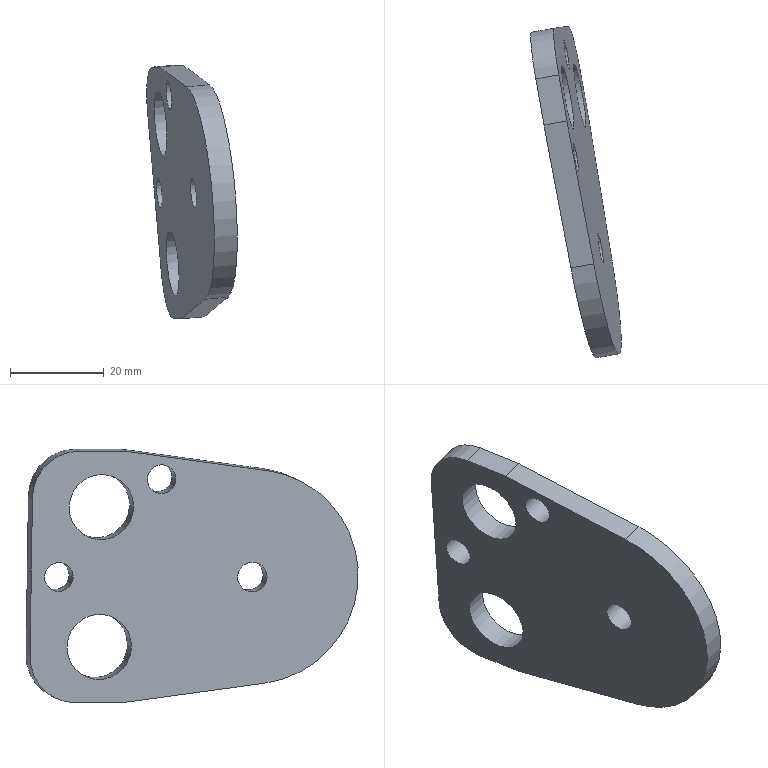Part | NX | features solid 2 | 1 solid | 15 faces | box 19.355 x 71.047 x 54.23 mm | volume 14370 mm3 | cylinder 8 | plane 7 | commonest cylinder face diameters 6.2 x2 14 x2 20 x2 6.4 x1 46 x1
STEP:
#1=CARTESIAN_POINT('',(1568.653,611.082,44.014));
#2=VERTEX_POINT('',#1);
#3=CARTESIAN_POINT('',(1567.775,621.082,34.053));
#4=VERTEX_POINT('',#3);
#5=CARTESIAN_POINT('',(1569.511,611.234,34.053));
#6=DIRECTION('',(-0.9811,-0.173,-0.08716));
#7=DIRECTION('',(-0.1736,0.9848,0.));
#8=AXIS2_PLACEMENT_3D('',#5,#6,#7);
#9=CIRCLE('',#8,10.);
#10=EDGE_CURVE('',#2,#4,#9,.T.);
#11=ORIENTED_EDGE('',*,*,#10,.F.);
#12=CARTESIAN_POINT('',(1573.558,611.947,44.45));
#13=VERTEX_POINT('',#12);
#14=CARTESIAN_POINT('',(1573.558,611.947,44.45));
#15=DIRECTION('',(-0.9811,-0.173,-0.08716));
#16=VECTOR('',#15,1000.);
#17=LINE('',#14,#16);
#18=EDGE_CURVE('',#13,#2,#17,.T.);
#19=ORIENTED_EDGE('',*,*,#18,.F.);
#20=CARTESIAN_POINT('',(1572.68,621.947,34.488));
#21=VERTEX_POINT('',#20);
#22=CARTESIAN_POINT('',(1574.416,612.099,34.488));
#23=DIRECTION('',(-0.9811,-0.173,-0.08716));
#24=DIRECTION('',(-0.1736,0.9848,0.));
#25=AXIS2_PLACEMENT_3D('',#22,#23,#24);
#26=CIRCLE('',#25,10.);
#27=EDGE_CURVE('',#13,#21,#26,.T.);
#28=ORIENTED_EDGE('',*,*,#27,.T.);
#29=CARTESIAN_POINT('',(1572.68,621.947,34.488));
#30=DIRECTION('',(-0.9811,-0.173,-0.08716));
#31=VECTOR('',#30,1000.);
#32=LINE('',#29,#31);
#33=EDGE_CURVE('',#21,#4,#32,.T.);
#34=ORIENTED_EDGE('',*,*,#33,.T.);
#35=EDGE_LOOP('',(#11,#19,#28,#34));
#36=FACE_BOUND('',#35,.T.);
#37=CARTESIAN_POINT('',(1574.416,612.099,34.488));
#38=DIRECTION('',(-0.9811,-0.173,-0.08716));
#39=DIRECTION('',(-0.1736,0.9848,0.));
#40=AXIS2_PLACEMENT_3D('',#37,#38,#39);
#41=CYLINDRICAL_SURFACE('',#40,10.);
#42=ADVANCED_FACE('',(#36),#41,.T.);
#43=CARTESIAN_POINT('',(1570.693,621.596,0.1819));
#44=VERTEX_POINT('',#43);
#45=CARTESIAN_POINT('',(1570.693,621.596,0.1819));
#46=DIRECTION('',(-0.08583,-0.01513,0.9962));
#47=VECTOR('',#46,1000.);
#48=LINE('',#45,#47);
#49=EDGE_CURVE('',#44,#4,#48,.T.);
#50=ORIENTED_EDGE('',*,*,#49,.T.);
#51=ORIENTED_EDGE('',*,*,#33,.F.);
#52=CARTESIAN_POINT('',(1575.598,622.461,0.6177));
#53=VERTEX_POINT('',#52);
#54=CARTESIAN_POINT('',(1575.598,622.461,0.6177));
#55=DIRECTION('',(-0.08583,-0.01513,0.9962));
#56=VECTOR('',#55,1000.);
#57=LINE('',#54,#56);
#58=EDGE_CURVE('',#53,#21,#57,.T.);
#59=ORIENTED_EDGE('',*,*,#58,.F.);
#60=CARTESIAN_POINT('',(1575.598,622.461,0.6177));
#61=DIRECTION('',(-0.9811,-0.173,-0.08716));
#62=VECTOR('',#61,1000.);
#63=LINE('',#60,#62);
#64=EDGE_CURVE('',#53,#44,#63,.T.);
#65=ORIENTED_EDGE('',*,*,#64,.T.);
#66=EDGE_LOOP('',(#50,#51,#59,#65));
#67=FACE_BOUND('',#66,.T.);
#68=CARTESIAN_POINT('',(1575.598,622.461,0.6177));
#69=DIRECTION('',(0.1736,-0.9848,0.));
#70=DIRECTION('',(0.08583,0.01513,-0.9962));
#71=AXIS2_PLACEMENT_3D('',#68,#69,#70);
#72=PLANE('',#71);
#73=ADVANCED_FACE('',(#67),#72,.F.);
#74=CARTESIAN_POINT('',(1573.288,611.9,-9.78));
#75=VERTEX_POINT('',#74);
#76=CARTESIAN_POINT('',(1572.429,611.748,0.1819));
#77=DIRECTION('',(-0.9811,-0.173,-0.08716));
#78=DIRECTION('',(-0.1736,0.9848,0.));
#79=AXIS2_PLACEMENT_3D('',#76,#77,#78);
#80=CIRCLE('',#79,10.);
#81=EDGE_CURVE('',#44,#75,#80,.T.);
#82=ORIENTED_EDGE('',*,*,#81,.F.);
#83=ORIENTED_EDGE('',*,*,#64,.F.);
#84=CARTESIAN_POINT('',(1578.193,612.764,-9.344));
#85=VERTEX_POINT('',#84);
#86=CARTESIAN_POINT('',(1577.335,612.613,0.6177));
#87=DIRECTION('',(-0.9811,-0.173,-0.08716));
#88=DIRECTION('',(-0.1736,0.9848,0.));
#89=AXIS2_PLACEMENT_3D('',#86,#87,#88);
#90=CIRCLE('',#89,10.);
#91=EDGE_CURVE('',#53,#85,#90,.T.);
#92=ORIENTED_EDGE('',*,*,#91,.T.);
#93=CARTESIAN_POINT('',(1578.193,612.764,-9.344));
#94=DIRECTION('',(-0.9811,-0.173,-0.08716));
#95=VECTOR('',#94,1000.);
#96=LINE('',#93,#95);
#97=EDGE_CURVE('',#85,#75,#96,.T.);
#98=ORIENTED_EDGE('',*,*,#97,.T.);
#99=EDGE_LOOP('',(#82,#83,#92,#98));
#100=FACE_BOUND('',#99,.T.);
#101=CARTESIAN_POINT('',(1577.335,612.613,0.6177));
#102=DIRECTION('',(-0.9811,-0.173,-0.08716));
#103=DIRECTION('',(-0.1736,0.9848,0.));
#104=AXIS2_PLACEMENT_3D('',#101,#102,#103);
#105=CYLINDRICAL_SURFACE('',#104,10.);
#106=ADVANCED_FACE('',(#100),#105,.T.);
#107=CARTESIAN_POINT('',(1575.024,602.051,-9.78));
#108=VERTEX_POINT('',#107);
#109=CARTESIAN_POINT('',(1575.024,602.051,-9.78));
#110=DIRECTION('',(-0.1736,0.9848,0.));
#111=VECTOR('',#110,1000.);
#112=LINE('',#109,#111);
#113=EDGE_CURVE('',#108,#75,#112,.T.);
#114=ORIENTED_EDGE('',*,*,#113,.T.);
#115=ORIENTED_EDGE('',*,*,#97,.F.);
#116=CARTESIAN_POINT('',(1579.929,602.916,-9.344));
#117=VERTEX_POINT('',#116);
#118=CARTESIAN_POINT('',(1579.929,602.916,-9.344));
#119=DIRECTION('',(-0.1736,0.9848,0.));
#120=VECTOR('',#119,1000.);
#121=LINE('',#118,#120);
#122=EDGE_CURVE('',#117,#85,#121,.T.);
#123=ORIENTED_EDGE('',*,*,#122,.F.);
#124=CARTESIAN_POINT('',(1579.929,602.916,-9.344));
#125=DIRECTION('',(-0.9811,-0.173,-0.08716));
#126=VECTOR('',#125,1000.);
#127=LINE('',#124,#126);
#128=EDGE_CURVE('',#117,#108,#127,.T.);
#129=ORIENTED_EDGE('',*,*,#128,.T.);
#130=EDGE_LOOP('',(#114,#115,#123,#129));
#131=FACE_BOUND('',#130,.T.);
#132=CARTESIAN_POINT('',(1579.929,602.916,-9.344));
#133=DIRECTION('',(-0.08583,-0.01513,0.9962));
#134=DIRECTION('',(0.1736,-0.9848,0.));
#135=AXIS2_PLACEMENT_3D('',#132,#133,#134);
#136=PLANE('',#135);
#137=ADVANCED_FACE('',(#131),#136,.F.);
#138=CARTESIAN_POINT('',(1580.061,571.375,-5.588));
#139=VERTEX_POINT('',#138);
#140=CARTESIAN_POINT('',(1580.061,571.375,-5.588));
#141=DIRECTION('',(-0.1606,0.9779,-0.1336));
#142=VECTOR('',#141,1000.);
#143=LINE('',#140,#142);
#144=EDGE_CURVE('',#139,#108,#143,.T.);
#145=ORIENTED_EDGE('',*,*,#144,.T.);
#146=ORIENTED_EDGE('',*,*,#128,.F.);
#147=CARTESIAN_POINT('',(1584.966,572.24,-5.152));
#148=VERTEX_POINT('',#147);
#149=CARTESIAN_POINT('',(1584.966,572.24,-5.152));
#150=DIRECTION('',(-0.1606,0.9779,-0.1336));
#151=VECTOR('',#150,1000.);
#152=LINE('',#149,#151);
#153=EDGE_CURVE('',#148,#117,#152,.T.);
#154=ORIENTED_EDGE('',*,*,#153,.F.);
#155=CARTESIAN_POINT('',(1584.966,572.24,-5.152));
#156=DIRECTION('',(-0.9811,-0.173,-0.08716));
#157=VECTOR('',#156,1000.);
#158=LINE('',#155,#157);
#159=EDGE_CURVE('',#148,#139,#158,.T.);
#160=ORIENTED_EDGE('',*,*,#159,.T.);
#161=EDGE_LOOP('',(#145,#146,#154,#160));
#162=FACE_BOUND('',#161,.T.);
#163=CARTESIAN_POINT('',(1584.966,572.24,-5.152));
#164=DIRECTION('',(-0.1083,0.1171,0.9872));
#165=DIRECTION('',(0.1606,-0.9779,0.1336));
#166=AXIS2_PLACEMENT_3D('',#163,#164,#165);
#167=PLANE('',#166);
#168=ADVANCED_FACE('',(#162),#167,.F.);
#169=CARTESIAN_POINT('',(1576.148,570.685,39.823));
#170=VERTEX_POINT('',#169);
#171=CARTESIAN_POINT('',(1577.569,574.068,17.117));
#172=DIRECTION('',(-0.9811,-0.173,-0.08716));
#173=DIRECTION('',(-0.1736,0.9848,0.));
#174=AXIS2_PLACEMENT_3D('',#171,#172,#173);
#175=CIRCLE('',#174,23.);
#176=EDGE_CURVE('',#139,#170,#175,.T.);
#177=ORIENTED_EDGE('',*,*,#176,.F.);
#178=ORIENTED_EDGE('',*,*,#159,.F.);
#179=CARTESIAN_POINT('',(1581.054,571.55,40.258));
#180=VERTEX_POINT('',#179);
#181=CARTESIAN_POINT('',(1582.474,574.933,17.553));
#182=DIRECTION('',(-0.9811,-0.173,-0.08716));
#183=DIRECTION('',(-0.1736,0.9848,0.));
#184=AXIS2_PLACEMENT_3D('',#181,#182,#183);
#185=CIRCLE('',#184,23.);
#186=EDGE_CURVE('',#148,#180,#185,.T.);
#187=ORIENTED_EDGE('',*,*,#186,.T.);
#188=CARTESIAN_POINT('',(1581.054,571.55,40.258));
#189=DIRECTION('',(-0.9811,-0.173,-0.08716));
#190=VECTOR('',#189,1000.);
#191=LINE('',#188,#190);
#192=EDGE_CURVE('',#180,#170,#191,.T.);
#193=ORIENTED_EDGE('',*,*,#192,.T.);
#194=EDGE_LOOP('',(#177,#178,#187,#193));
#195=FACE_BOUND('',#194,.T.);
#196=CARTESIAN_POINT('',(1582.474,574.933,17.553));
#197=DIRECTION('',(-0.9811,-0.173,-0.08716));
#198=DIRECTION('',(-0.1736,0.9848,0.));
#199=AXIS2_PLACEMENT_3D('',#196,#197,#198);
#200=CYLINDRICAL_SURFACE('',#199,23.);
#201=ADVANCED_FACE('',(#195),#200,.T.);
#202=CARTESIAN_POINT('',(1570.389,601.234,44.014));
#203=VERTEX_POINT('',#202);
#204=CARTESIAN_POINT('',(1576.148,570.685,39.823));
#205=DIRECTION('',(-0.1836,0.9739,0.1336));
#206=VECTOR('',#205,1000.);
#207=LINE('',#204,#206);
#208=EDGE_CURVE('',#170,#203,#207,.T.);
#209=ORIENTED_EDGE('',*,*,#208,.F.);
#210=ORIENTED_EDGE('',*,*,#192,.F.);
#211=CARTESIAN_POINT('',(1575.295,602.099,44.45));
#212=VERTEX_POINT('',#211);
#213=CARTESIAN_POINT('',(1581.054,571.55,40.258));
#214=DIRECTION('',(-0.1836,0.9739,0.1336));
#215=VECTOR('',#214,1000.);
#216=LINE('',#213,#215);
#217=EDGE_CURVE('',#180,#212,#216,.T.);
#218=ORIENTED_EDGE('',*,*,#217,.T.);
#219=CARTESIAN_POINT('',(1575.295,602.099,44.45));
#220=DIRECTION('',(-0.9811,-0.173,-0.08716));
#221=VECTOR('',#220,1000.);
#222=LINE('',#219,#221);
#223=EDGE_CURVE('',#212,#203,#222,.T.);
#224=ORIENTED_EDGE('',*,*,#223,.T.);
#225=EDGE_LOOP('',(#209,#210,#218,#224));
#226=FACE_BOUND('',#225,.T.);
#227=CARTESIAN_POINT('',(1581.054,571.55,40.258));
#228=DIRECTION('',(-0.06176,-0.1471,0.9872));
#229=DIRECTION('',(0.1836,-0.9739,-0.1336));
#230=AXIS2_PLACEMENT_3D('',#227,#228,#229);
#231=PLANE('',#230);
#232=ADVANCED_FACE('',(#226),#231,.T.);
#233=CARTESIAN_POINT('',(1570.389,601.234,44.014));
#234=DIRECTION('',(-0.1736,0.9848,0.));
#235=VECTOR('',#234,1000.);
#236=LINE('',#233,#235);
#237=EDGE_CURVE('',#203,#2,#236,.T.);
#238=ORIENTED_EDGE('',*,*,#237,.F.);
#239=ORIENTED_EDGE('',*,*,#223,.F.);
#240=CARTESIAN_POINT('',(1575.295,602.099,44.45));
#241=DIRECTION('',(-0.1736,0.9848,0.));
#242=VECTOR('',#241,1000.);
#243=LINE('',#240,#242);
#244=EDGE_CURVE('',#212,#13,#243,.T.);
#245=ORIENTED_EDGE('',*,*,#244,.T.);
#246=ORIENTED_EDGE('',*,*,#18,.T.);
#247=EDGE_LOOP('',(#238,#239,#245,#246));
#248=FACE_BOUND('',#247,.T.);
#249=CARTESIAN_POINT('',(1575.295,602.099,44.45));
#250=DIRECTION('',(-0.08583,-0.01513,0.9962));
#251=DIRECTION('',(0.1736,-0.9848,0.));
#252=AXIS2_PLACEMENT_3D('',#249,#250,#251);
#253=PLANE('',#252);
#254=ADVANCED_FACE('',(#248),#253,.T.);
#255=CARTESIAN_POINT('',(1576.816,614.552,2.61));
#256=VERTEX_POINT('',#255);
#257=CARTESIAN_POINT('',(1578.031,607.659,2.61));
#258=DIRECTION('',(-0.9811,-0.173,-0.08716));
#259=DIRECTION('',(-0.1736,0.9848,0.));
#260=AXIS2_PLACEMENT_3D('',#257,#258,#259);
#261=CIRCLE('',#260,7.);
#262=EDGE_CURVE('',#256,#256,#261,.T.);
#263=ORIENTED_EDGE('',*,*,#262,.T.);
#264=EDGE_LOOP('',(#263));
#265=FACE_BOUND('',#264,.T.);
#266=CARTESIAN_POINT('',(1574.241,614.098,32.496));
#267=VERTEX_POINT('',#266);
#268=CARTESIAN_POINT('',(1575.456,607.205,32.496));
#269=DIRECTION('',(-0.9811,-0.173,-0.08716));
#270=DIRECTION('',(-0.1736,0.9848,0.));
#271=AXIS2_PLACEMENT_3D('',#268,#269,#270);
#272=CIRCLE('',#271,7.);
#273=EDGE_CURVE('',#267,#267,#272,.T.);
#274=ORIENTED_EDGE('',*,*,#273,.T.);
#275=EDGE_LOOP('',(#274));
#276=FACE_BOUND('',#275,.T.);
#277=CARTESIAN_POINT('',(1581.918,578.085,17.553));
#278=VERTEX_POINT('',#277);
#279=CARTESIAN_POINT('',(1582.474,574.933,17.553));
#280=DIRECTION('',(-0.9811,-0.173,-0.08716));
#281=DIRECTION('',(-0.1736,0.9848,0.));
#282=AXIS2_PLACEMENT_3D('',#279,#280,#281);
#283=CIRCLE('',#282,3.2);
#284=EDGE_CURVE('',#278,#278,#283,.T.);
#285=ORIENTED_EDGE('',*,*,#284,.T.);
#286=EDGE_LOOP('',(#285));
#287=FACE_BOUND('',#286,.T.);
#288=CARTESIAN_POINT('',(1576.66,597.364,38.473));
#289=VERTEX_POINT('',#288);
#290=CARTESIAN_POINT('',(1577.199,594.311,38.473));
#291=DIRECTION('',(-0.9811,-0.173,-0.08716));
#292=DIRECTION('',(-0.1736,0.9848,0.));
#293=AXIS2_PLACEMENT_3D('',#290,#291,#292);
#294=CIRCLE('',#293,3.1);
#295=EDGE_CURVE('',#289,#289,#294,.T.);
#296=ORIENTED_EDGE('',*,*,#295,.T.);
#297=EDGE_LOOP('',(#296));
#298=FACE_BOUND('',#297,.T.);
#299=CARTESIAN_POINT('',(1574.643,619.348,17.553));
#300=VERTEX_POINT('',#299);
#301=CARTESIAN_POINT('',(1575.181,616.295,17.553));
#302=DIRECTION('',(-0.9811,-0.173,-0.08716));
#303=DIRECTION('',(-0.1736,0.9848,0.));
#304=AXIS2_PLACEMENT_3D('',#301,#302,#303);
#305=CIRCLE('',#304,3.1);
#306=EDGE_CURVE('',#300,#300,#305,.T.);
#307=ORIENTED_EDGE('',*,*,#306,.T.);
#308=EDGE_LOOP('',(#307));
#309=FACE_BOUND('',#308,.T.);
#310=ORIENTED_EDGE('',*,*,#27,.F.);
#311=ORIENTED_EDGE('',*,*,#244,.F.);
#312=ORIENTED_EDGE('',*,*,#217,.F.);
#313=ORIENTED_EDGE('',*,*,#186,.F.);
#314=ORIENTED_EDGE('',*,*,#153,.T.);
#315=ORIENTED_EDGE('',*,*,#122,.T.);
#316=ORIENTED_EDGE('',*,*,#91,.F.);
#317=ORIENTED_EDGE('',*,*,#58,.T.);
#318=EDGE_LOOP('',(#310,#311,#312,#313,#314,#315,#316,#317));
#319=FACE_BOUND('',#318,.T.);
#320=CARTESIAN_POINT('',(1574.416,612.099,34.488));
#321=DIRECTION('',(-0.9811,-0.173,-0.08716));
#322=DIRECTION('',(-0.1736,0.9848,0.));
#323=AXIS2_PLACEMENT_3D('',#320,#321,#322);
#324=PLANE('',#323);
#325=ADVANCED_FACE('',(#265,#276,#287,#298,#309,#319),#324,.F.);
#326=CARTESIAN_POINT('',(1571.91,613.688,2.174));
#327=VERTEX_POINT('',#326);
#328=CARTESIAN_POINT('',(1573.126,606.794,2.174));
#329=DIRECTION('',(-0.9811,-0.173,-0.08716));
#330=DIRECTION('',(-0.1736,0.9848,0.));
#331=AXIS2_PLACEMENT_3D('',#328,#329,#330);
#332=CIRCLE('',#331,7.);
#333=EDGE_CURVE('',#327,#327,#332,.T.);
#334=ORIENTED_EDGE('',*,*,#333,.F.);
#335=EDGE_LOOP('',(#334));
#336=FACE_BOUND('',#335,.T.);
#337=CARTESIAN_POINT('',(1569.335,613.233,32.06));
#338=VERTEX_POINT('',#337);
#339=CARTESIAN_POINT('',(1570.551,606.34,32.06));
#340=DIRECTION('',(-0.9811,-0.173,-0.08716));
#341=DIRECTION('',(-0.1736,0.9848,0.));
#342=AXIS2_PLACEMENT_3D('',#339,#340,#341);
#343=CIRCLE('',#342,7.);
#344=EDGE_CURVE('',#338,#338,#343,.T.);
#345=ORIENTED_EDGE('',*,*,#344,.F.);
#346=EDGE_LOOP('',(#345));
#347=FACE_BOUND('',#346,.T.);
#348=CARTESIAN_POINT('',(1577.013,577.22,17.117));
#349=VERTEX_POINT('',#348);
#350=CARTESIAN_POINT('',(1577.569,574.068,17.117));
#351=DIRECTION('',(-0.9811,-0.173,-0.08716));
#352=DIRECTION('',(-0.1736,0.9848,0.));
#353=AXIS2_PLACEMENT_3D('',#350,#351,#352);
#354=CIRCLE('',#353,3.2);
#355=EDGE_CURVE('',#349,#349,#354,.T.);
#356=ORIENTED_EDGE('',*,*,#355,.F.);
#357=EDGE_LOOP('',(#356));
#358=FACE_BOUND('',#357,.T.);
#359=CARTESIAN_POINT('',(1571.755,596.499,38.037));
#360=VERTEX_POINT('',#359);
#361=CARTESIAN_POINT('',(1572.293,593.447,38.037));
#362=DIRECTION('',(-0.9811,-0.173,-0.08716));
#363=DIRECTION('',(-0.1736,0.9848,0.));
#364=AXIS2_PLACEMENT_3D('',#361,#362,#363);
#365=CIRCLE('',#364,3.1);
#366=EDGE_CURVE('',#360,#360,#365,.T.);
#367=ORIENTED_EDGE('',*,*,#366,.F.);
#368=EDGE_LOOP('',(#367));
#369=FACE_BOUND('',#368,.T.);
#370=CARTESIAN_POINT('',(1569.737,618.483,17.117));
#371=VERTEX_POINT('',#370);
#372=CARTESIAN_POINT('',(1570.276,615.43,17.117));
#373=DIRECTION('',(-0.9811,-0.173,-0.08716));
#374=DIRECTION('',(-0.1736,0.9848,0.));
#375=AXIS2_PLACEMENT_3D('',#372,#373,#374);
#376=CIRCLE('',#375,3.1);
#377=EDGE_CURVE('',#371,#371,#376,.T.);
#378=ORIENTED_EDGE('',*,*,#377,.F.);
#379=EDGE_LOOP('',(#378));
#380=FACE_BOUND('',#379,.T.);
#381=ORIENTED_EDGE('',*,*,#10,.T.);
#382=ORIENTED_EDGE('',*,*,#49,.F.);
#383=ORIENTED_EDGE('',*,*,#81,.T.);
#384=ORIENTED_EDGE('',*,*,#113,.F.);
#385=ORIENTED_EDGE('',*,*,#144,.F.);
#386=ORIENTED_EDGE('',*,*,#176,.T.);
#387=ORIENTED_EDGE('',*,*,#208,.T.);
#388=ORIENTED_EDGE('',*,*,#237,.T.);
#389=EDGE_LOOP('',(#381,#382,#383,#384,#385,#386,#387,#388));
#390=FACE_BOUND('',#389,.T.);
#391=CARTESIAN_POINT('',(1569.511,611.234,34.053));
#392=DIRECTION('',(-0.9811,-0.173,-0.08716));
#393=DIRECTION('',(-0.1736,0.9848,0.));
#394=AXIS2_PLACEMENT_3D('',#391,#392,#393);
#395=PLANE('',#394);
#396=ADVANCED_FACE('',(#336,#347,#358,#369,#380,#390),#395,.T.);
#397=ORIENTED_EDGE('',*,*,#377,.T.);
#398=EDGE_LOOP('',(#397));
#399=FACE_BOUND('',#398,.T.);
#400=ORIENTED_EDGE('',*,*,#306,.F.);
#401=EDGE_LOOP('',(#400));
#402=FACE_BOUND('',#401,.T.);
#403=CARTESIAN_POINT('',(1575.181,616.295,17.553));
#404=DIRECTION('',(-0.9811,-0.173,-0.08716));
#405=DIRECTION('',(-0.1736,0.9848,0.));
#406=AXIS2_PLACEMENT_3D('',#403,#404,#405);
#407=CYLINDRICAL_SURFACE('',#406,3.1);
#408=ADVANCED_FACE('',(#399,#402),#407,.F.);
#409=ORIENTED_EDGE('',*,*,#366,.T.);
#410=EDGE_LOOP('',(#409));
#411=FACE_BOUND('',#410,.T.);
#412=ORIENTED_EDGE('',*,*,#295,.F.);
#413=EDGE_LOOP('',(#412));
#414=FACE_BOUND('',#413,.T.);
#415=CARTESIAN_POINT('',(1577.199,594.311,38.473));
#416=DIRECTION('',(-0.9811,-0.173,-0.08716));
#417=DIRECTION('',(-0.1736,0.9848,0.));
#418=AXIS2_PLACEMENT_3D('',#415,#416,#417);
#419=CYLINDRICAL_SURFACE('',#418,3.1);
#420=ADVANCED_FACE('',(#411,#414),#419,.F.);
#421=ORIENTED_EDGE('',*,*,#355,.T.);
#422=EDGE_LOOP('',(#421));
#423=FACE_BOUND('',#422,.T.);
#424=ORIENTED_EDGE('',*,*,#284,.F.);
#425=EDGE_LOOP('',(#424));
#426=FACE_BOUND('',#425,.T.);
#427=CARTESIAN_POINT('',(1582.474,574.933,17.553));
#428=DIRECTION('',(-0.9811,-0.173,-0.08716));
#429=DIRECTION('',(-0.1736,0.9848,0.));
#430=AXIS2_PLACEMENT_3D('',#427,#428,#429);
#431=CYLINDRICAL_SURFACE('',#430,3.2);
#432=ADVANCED_FACE('',(#423,#426),#431,.F.);
#433=ORIENTED_EDGE('',*,*,#344,.T.);
#434=EDGE_LOOP('',(#433));
#435=FACE_BOUND('',#434,.T.);
#436=ORIENTED_EDGE('',*,*,#273,.F.);
#437=EDGE_LOOP('',(#436));
#438=FACE_BOUND('',#437,.T.);
#439=CARTESIAN_POINT('',(1575.456,607.205,32.496));
#440=DIRECTION('',(-0.9811,-0.173,-0.08716));
#441=DIRECTION('',(-0.1736,0.9848,0.));
#442=AXIS2_PLACEMENT_3D('',#439,#440,#441);
#443=CYLINDRICAL_SURFACE('',#442,7.);
#444=ADVANCED_FACE('',(#435,#438),#443,.F.);
#445=ORIENTED_EDGE('',*,*,#333,.T.);
#446=EDGE_LOOP('',(#445));
#447=FACE_BOUND('',#446,.T.);
#448=ORIENTED_EDGE('',*,*,#262,.F.);
#449=EDGE_LOOP('',(#448));
#450=FACE_BOUND('',#449,.T.);
#451=CARTESIAN_POINT('',(1578.031,607.659,2.61));
#452=DIRECTION('',(-0.9811,-0.173,-0.08716));
#453=DIRECTION('',(-0.1736,0.9848,0.));
#454=AXIS2_PLACEMENT_3D('',#451,#452,#453);
#455=CYLINDRICAL_SURFACE('',#454,7.);
#456=ADVANCED_FACE('',(#447,#450),#455,.F.);
#457=CLOSED_SHELL('',(#42,#73,#106,#137,#168,#201,#232,#254,#325,#396,#408,#420,#432,#444,#456));
#458=MANIFOLD_SOLID_BREP('',#457);
#459=(LENGTH_UNIT()NAMED_UNIT(*)SI_UNIT(.MILLI.,.METRE.));
#460=UNCERTAINTY_MEASURE_WITH_UNIT(LENGTH_MEASURE(0.00001),#459,'','');
#461=(NAMED_UNIT(*)PLANE_ANGLE_UNIT()SI_UNIT($,.RADIAN.));
#462=(NAMED_UNIT(*)SI_UNIT($,.STERADIAN.)SOLID_ANGLE_UNIT());
#463=(GEOMETRIC_REPRESENTATION_CONTEXT(3)GLOBAL_UNCERTAINTY_ASSIGNED_CONTEXT((#460))GLOBAL_UNIT_ASSIGNED_CONTEXT((#459,#461,#462))REPRESENTATION_CONTEXT('',''));
#464=ADVANCED_BREP_SHAPE_REPRESENTATION('',(#458),#463);